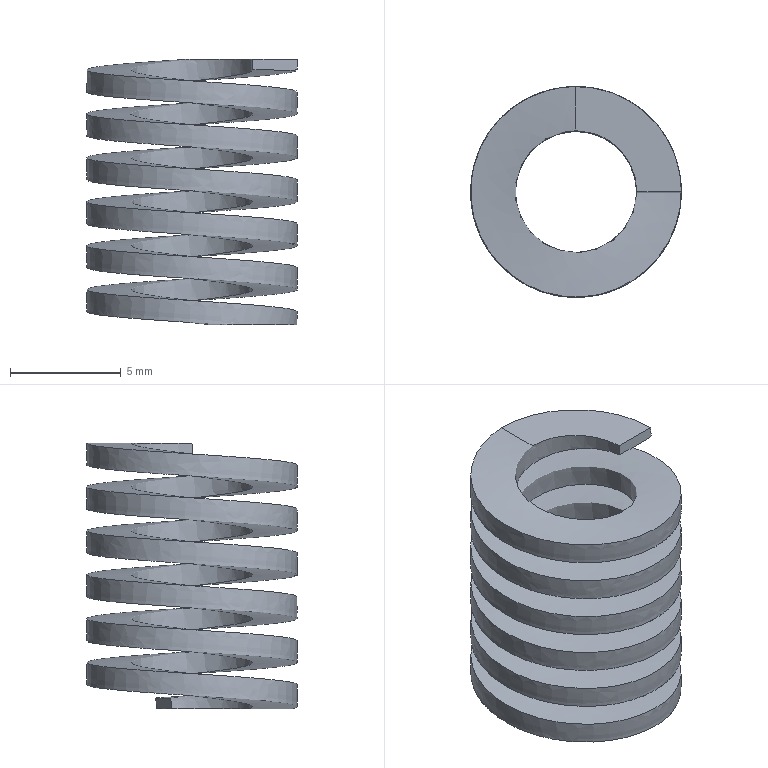Part | Creo | 1 solid | 6 faces | box 9.519 x 9.516 x 12 mm | volume 277.986 mm3 | plane 4 | spline 2